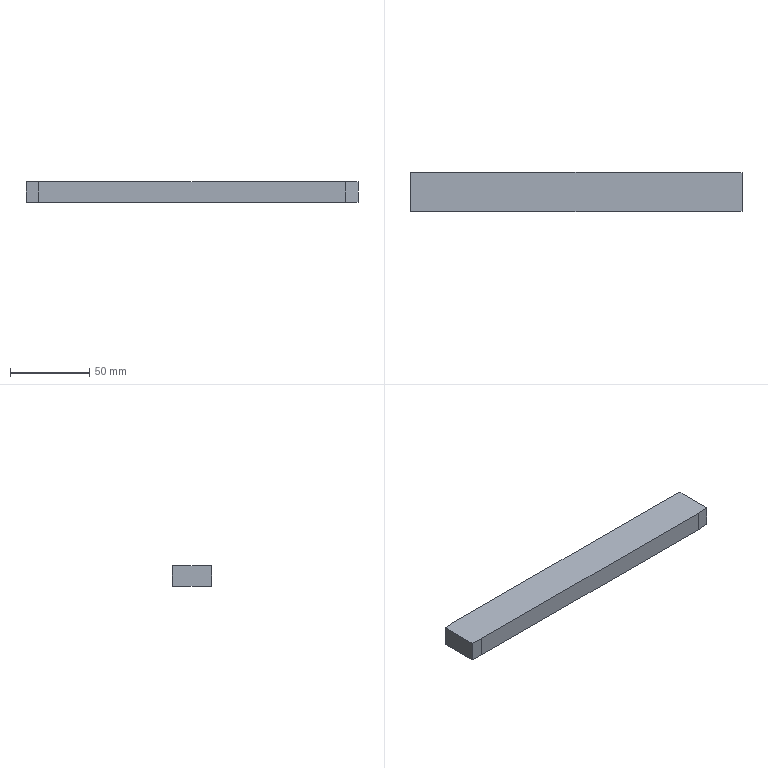Part | SolidWorks | features Cut 1, Extrusion 1 | 1 solid | 10 faces | box 209.55 x 25 x 12.7 mm | volume 66431 mm3 | plane 10
STEP:
#1=CARTESIAN_POINT('',(-104.775,12.,-6.35));
#2=VERTEX_POINT('',#1);
#3=CARTESIAN_POINT('',(-104.775,-12.,-6.35));
#4=VERTEX_POINT('',#3);
#5=CARTESIAN_POINT('',(-104.775,12.5,-6.35));
#6=DIRECTION('',(0.,-1.,0.));
#7=VECTOR('',#6,1000.);
#8=LINE('',#5,#7);
#9=EDGE_CURVE('',#2,#4,#8,.T.);
#10=ORIENTED_EDGE('',*,*,#9,.T.);
#11=CARTESIAN_POINT('',(-104.775,-12.,6.35));
#12=VERTEX_POINT('',#11);
#13=CARTESIAN_POINT('',(-104.775,-12.,-6.35));
#14=DIRECTION('',(0.,0.,1.));
#15=VECTOR('',#14,1000.);
#16=LINE('',#13,#15);
#17=EDGE_CURVE('',#4,#12,#16,.T.);
#18=ORIENTED_EDGE('',*,*,#17,.T.);
#19=CARTESIAN_POINT('',(-104.775,12.,6.35));
#20=VERTEX_POINT('',#19);
#21=CARTESIAN_POINT('',(-104.775,12.5,6.35));
#22=DIRECTION('',(0.,-1.,0.));
#23=VECTOR('',#22,1000.);
#24=LINE('',#21,#23);
#25=EDGE_CURVE('',#20,#12,#24,.T.);
#26=ORIENTED_EDGE('',*,*,#25,.F.);
#27=CARTESIAN_POINT('',(-104.775,12.,-6.35));
#28=DIRECTION('',(0.,0.,1.));
#29=VECTOR('',#28,1000.);
#30=LINE('',#27,#29);
#31=EDGE_CURVE('',#2,#20,#30,.T.);
#32=ORIENTED_EDGE('',*,*,#31,.F.);
#33=EDGE_LOOP('',(#10,#18,#26,#32));
#34=FACE_OUTER_BOUND('',#33,.T.);
#35=CARTESIAN_POINT('',(-104.775,12.5,6.35));
#36=DIRECTION('',(1.,0.,0.));
#37=DIRECTION('',(0.,0.,-1.));
#38=AXIS2_PLACEMENT_3D('',#35,#36,#37);
#39=PLANE('',#38);
#40=ADVANCED_FACE('',(#34),#39,.F.);
#41=CARTESIAN_POINT('',(-96.775,-12.5,6.35));
#42=VERTEX_POINT('',#41);
#43=CARTESIAN_POINT('',(96.775,-12.5,6.35));
#44=VERTEX_POINT('',#43);
#45=CARTESIAN_POINT('',(-104.775,-12.5,6.35));
#46=DIRECTION('',(1.,0.,0.));
#47=VECTOR('',#46,1000.);
#48=LINE('',#45,#47);
#49=EDGE_CURVE('',#42,#44,#48,.T.);
#50=ORIENTED_EDGE('',*,*,#49,.F.);
#51=CARTESIAN_POINT('',(-96.775,-12.5,-6.35));
#52=VERTEX_POINT('',#51);
#53=CARTESIAN_POINT('',(-96.775,-12.5,-6.35));
#54=DIRECTION('',(0.,0.,1.));
#55=VECTOR('',#54,1000.);
#56=LINE('',#53,#55);
#57=EDGE_CURVE('',#52,#42,#56,.T.);
#58=ORIENTED_EDGE('',*,*,#57,.F.);
#59=CARTESIAN_POINT('',(96.775,-12.5,-6.35));
#60=VERTEX_POINT('',#59);
#61=CARTESIAN_POINT('',(-104.775,-12.5,-6.35));
#62=DIRECTION('',(1.,0.,0.));
#63=VECTOR('',#62,1000.);
#64=LINE('',#61,#63);
#65=EDGE_CURVE('',#52,#60,#64,.T.);
#66=ORIENTED_EDGE('',*,*,#65,.T.);
#67=CARTESIAN_POINT('',(96.775,-12.5,-6.35));
#68=DIRECTION('',(0.,0.,1.));
#69=VECTOR('',#68,1000.);
#70=LINE('',#67,#69);
#71=EDGE_CURVE('',#60,#44,#70,.T.);
#72=ORIENTED_EDGE('',*,*,#71,.T.);
#73=EDGE_LOOP('',(#50,#58,#66,#72));
#74=FACE_OUTER_BOUND('',#73,.T.);
#75=CARTESIAN_POINT('',(-104.775,-12.5,6.35));
#76=DIRECTION('',(0.,1.,0.));
#77=DIRECTION('',(-1.,0.,0.));
#78=AXIS2_PLACEMENT_3D('',#75,#76,#77);
#79=PLANE('',#78);
#80=ADVANCED_FACE('',(#74),#79,.F.);
#81=CARTESIAN_POINT('',(104.775,-12.,6.35));
#82=VERTEX_POINT('',#81);
#83=CARTESIAN_POINT('',(104.775,12.,6.35));
#84=VERTEX_POINT('',#83);
#85=CARTESIAN_POINT('',(104.775,12.5,6.35));
#86=DIRECTION('',(0.,1.,0.));
#87=VECTOR('',#86,1000.);
#88=LINE('',#85,#87);
#89=EDGE_CURVE('',#82,#84,#88,.T.);
#90=ORIENTED_EDGE('',*,*,#89,.F.);
#91=CARTESIAN_POINT('',(104.775,-12.,-6.35));
#92=VERTEX_POINT('',#91);
#93=CARTESIAN_POINT('',(104.775,-12.,-6.35));
#94=DIRECTION('',(0.,0.,1.));
#95=VECTOR('',#94,1000.);
#96=LINE('',#93,#95);
#97=EDGE_CURVE('',#92,#82,#96,.T.);
#98=ORIENTED_EDGE('',*,*,#97,.F.);
#99=CARTESIAN_POINT('',(104.775,12.,-6.35));
#100=VERTEX_POINT('',#99);
#101=CARTESIAN_POINT('',(104.775,12.5,-6.35));
#102=DIRECTION('',(0.,1.,0.));
#103=VECTOR('',#102,1000.);
#104=LINE('',#101,#103);
#105=EDGE_CURVE('',#92,#100,#104,.T.);
#106=ORIENTED_EDGE('',*,*,#105,.T.);
#107=CARTESIAN_POINT('',(104.775,12.,-6.35));
#108=DIRECTION('',(0.,0.,1.));
#109=VECTOR('',#108,1000.);
#110=LINE('',#107,#109);
#111=EDGE_CURVE('',#100,#84,#110,.T.);
#112=ORIENTED_EDGE('',*,*,#111,.T.);
#113=EDGE_LOOP('',(#90,#98,#106,#112));
#114=FACE_OUTER_BOUND('',#113,.T.);
#115=CARTESIAN_POINT('',(104.775,12.5,6.35));
#116=DIRECTION('',(-1.,0.,0.));
#117=DIRECTION('',(0.,0.,1.));
#118=AXIS2_PLACEMENT_3D('',#115,#116,#117);
#119=PLANE('',#118);
#120=ADVANCED_FACE('',(#114),#119,.F.);
#121=CARTESIAN_POINT('',(96.775,12.5,6.35));
#122=VERTEX_POINT('',#121);
#123=CARTESIAN_POINT('',(-96.775,12.5,6.35));
#124=VERTEX_POINT('',#123);
#125=CARTESIAN_POINT('',(-104.775,12.5,6.35));
#126=DIRECTION('',(-1.,0.,0.));
#127=VECTOR('',#126,1000.);
#128=LINE('',#125,#127);
#129=EDGE_CURVE('',#122,#124,#128,.T.);
#130=ORIENTED_EDGE('',*,*,#129,.F.);
#131=CARTESIAN_POINT('',(96.775,12.5,-6.35));
#132=VERTEX_POINT('',#131);
#133=CARTESIAN_POINT('',(96.775,12.5,-6.35));
#134=DIRECTION('',(0.,0.,1.));
#135=VECTOR('',#134,1000.);
#136=LINE('',#133,#135);
#137=EDGE_CURVE('',#132,#122,#136,.T.);
#138=ORIENTED_EDGE('',*,*,#137,.F.);
#139=CARTESIAN_POINT('',(-96.775,12.5,-6.35));
#140=VERTEX_POINT('',#139);
#141=CARTESIAN_POINT('',(-104.775,12.5,-6.35));
#142=DIRECTION('',(-1.,0.,0.));
#143=VECTOR('',#142,1000.);
#144=LINE('',#141,#143);
#145=EDGE_CURVE('',#132,#140,#144,.T.);
#146=ORIENTED_EDGE('',*,*,#145,.T.);
#147=CARTESIAN_POINT('',(-96.775,12.5,-6.35));
#148=DIRECTION('',(0.,0.,1.));
#149=VECTOR('',#148,1000.);
#150=LINE('',#147,#149);
#151=EDGE_CURVE('',#140,#124,#150,.T.);
#152=ORIENTED_EDGE('',*,*,#151,.T.);
#153=EDGE_LOOP('',(#130,#138,#146,#152));
#154=FACE_OUTER_BOUND('',#153,.T.);
#155=CARTESIAN_POINT('',(-104.775,12.5,6.35));
#156=DIRECTION('',(0.,-1.,0.));
#157=DIRECTION('',(1.,0.,0.));
#158=AXIS2_PLACEMENT_3D('',#155,#156,#157);
#159=PLANE('',#158);
#160=ADVANCED_FACE('',(#154),#159,.F.);
#161=CARTESIAN_POINT('',(-104.775,-12.,6.35));
#162=DIRECTION('',(-0.9981,0.06238,0.));
#163=VECTOR('',#162,1000.);
#164=LINE('',#161,#163);
#165=EDGE_CURVE('',#42,#12,#164,.T.);
#166=ORIENTED_EDGE('',*,*,#165,.F.);
#167=ORIENTED_EDGE('',*,*,#49,.T.);
#168=CARTESIAN_POINT('',(104.775,-12.,6.35));
#169=DIRECTION('',(-0.9981,-0.06238,0.));
#170=VECTOR('',#169,1000.);
#171=LINE('',#168,#170);
#172=EDGE_CURVE('',#82,#44,#171,.T.);
#173=ORIENTED_EDGE('',*,*,#172,.F.);
#174=ORIENTED_EDGE('',*,*,#89,.T.);
#175=CARTESIAN_POINT('',(104.775,12.,6.35));
#176=DIRECTION('',(0.9981,-0.06238,0.));
#177=VECTOR('',#176,1000.);
#178=LINE('',#175,#177);
#179=EDGE_CURVE('',#122,#84,#178,.T.);
#180=ORIENTED_EDGE('',*,*,#179,.F.);
#181=ORIENTED_EDGE('',*,*,#129,.T.);
#182=CARTESIAN_POINT('',(-104.775,12.,6.35));
#183=DIRECTION('',(0.9981,0.06238,0.));
#184=VECTOR('',#183,1000.);
#185=LINE('',#182,#184);
#186=EDGE_CURVE('',#20,#124,#185,.T.);
#187=ORIENTED_EDGE('',*,*,#186,.F.);
#188=ORIENTED_EDGE('',*,*,#25,.T.);
#189=EDGE_LOOP('',(#166,#167,#173,#174,#180,#181,#187,#188));
#190=FACE_OUTER_BOUND('',#189,.T.);
#191=CARTESIAN_POINT('',(-104.775,-12.5,6.35));
#192=DIRECTION('',(0.,0.,1.));
#193=DIRECTION('',(1.,0.,0.));
#194=AXIS2_PLACEMENT_3D('',#191,#192,#193);
#195=PLANE('',#194);
#196=ADVANCED_FACE('',(#190),#195,.T.);
#197=ORIENTED_EDGE('',*,*,#65,.F.);
#198=CARTESIAN_POINT('',(-104.775,-12.,-6.35));
#199=DIRECTION('',(-0.9981,0.06238,0.));
#200=VECTOR('',#199,1000.);
#201=LINE('',#198,#200);
#202=EDGE_CURVE('',#52,#4,#201,.T.);
#203=ORIENTED_EDGE('',*,*,#202,.T.);
#204=ORIENTED_EDGE('',*,*,#9,.F.);
#205=CARTESIAN_POINT('',(-104.775,12.,-6.35));
#206=DIRECTION('',(0.9981,0.06238,0.));
#207=VECTOR('',#206,1000.);
#208=LINE('',#205,#207);
#209=EDGE_CURVE('',#2,#140,#208,.T.);
#210=ORIENTED_EDGE('',*,*,#209,.T.);
#211=ORIENTED_EDGE('',*,*,#145,.F.);
#212=CARTESIAN_POINT('',(104.775,12.,-6.35));
#213=DIRECTION('',(0.9981,-0.06238,0.));
#214=VECTOR('',#213,1000.);
#215=LINE('',#212,#214);
#216=EDGE_CURVE('',#132,#100,#215,.T.);
#217=ORIENTED_EDGE('',*,*,#216,.T.);
#218=ORIENTED_EDGE('',*,*,#105,.F.);
#219=CARTESIAN_POINT('',(104.775,-12.,-6.35));
#220=DIRECTION('',(-0.9981,-0.06238,0.));
#221=VECTOR('',#220,1000.);
#222=LINE('',#219,#221);
#223=EDGE_CURVE('',#92,#60,#222,.T.);
#224=ORIENTED_EDGE('',*,*,#223,.T.);
#225=EDGE_LOOP('',(#197,#203,#204,#210,#211,#217,#218,#224));
#226=FACE_OUTER_BOUND('',#225,.T.);
#227=CARTESIAN_POINT('',(-104.775,-12.5,-6.35));
#228=DIRECTION('',(0.,0.,1.));
#229=DIRECTION('',(1.,0.,0.));
#230=AXIS2_PLACEMENT_3D('',#227,#228,#229);
#231=PLANE('',#230);
#232=ADVANCED_FACE('',(#226),#231,.F.);
#233=ORIENTED_EDGE('',*,*,#186,.T.);
#234=ORIENTED_EDGE('',*,*,#151,.F.);
#235=ORIENTED_EDGE('',*,*,#209,.F.);
#236=ORIENTED_EDGE('',*,*,#31,.T.);
#237=EDGE_LOOP('',(#233,#234,#235,#236));
#238=FACE_OUTER_BOUND('',#237,.T.);
#239=CARTESIAN_POINT('',(-104.775,12.,-6.35));
#240=DIRECTION('',(0.06238,-0.9981,0.));
#241=DIRECTION('',(0.9981,0.06238,0.));
#242=AXIS2_PLACEMENT_3D('',#239,#240,#241);
#243=PLANE('',#242);
#244=ADVANCED_FACE('',(#238),#243,.F.);
#245=ORIENTED_EDGE('',*,*,#179,.T.);
#246=ORIENTED_EDGE('',*,*,#111,.F.);
#247=ORIENTED_EDGE('',*,*,#216,.F.);
#248=ORIENTED_EDGE('',*,*,#137,.T.);
#249=EDGE_LOOP('',(#245,#246,#247,#248));
#250=FACE_OUTER_BOUND('',#249,.T.);
#251=CARTESIAN_POINT('',(104.775,12.,-6.35));
#252=DIRECTION('',(-0.06238,-0.9981,0.));
#253=DIRECTION('',(0.9981,-0.06238,0.));
#254=AXIS2_PLACEMENT_3D('',#251,#252,#253);
#255=PLANE('',#254);
#256=ADVANCED_FACE('',(#250),#255,.F.);
#257=ORIENTED_EDGE('',*,*,#172,.T.);
#258=ORIENTED_EDGE('',*,*,#71,.F.);
#259=ORIENTED_EDGE('',*,*,#223,.F.);
#260=ORIENTED_EDGE('',*,*,#97,.T.);
#261=EDGE_LOOP('',(#257,#258,#259,#260));
#262=FACE_OUTER_BOUND('',#261,.T.);
#263=CARTESIAN_POINT('',(104.775,-12.,-6.35));
#264=DIRECTION('',(-0.06238,0.9981,0.));
#265=DIRECTION('',(-0.9981,-0.06238,0.));
#266=AXIS2_PLACEMENT_3D('',#263,#264,#265);
#267=PLANE('',#266);
#268=ADVANCED_FACE('',(#262),#267,.F.);
#269=ORIENTED_EDGE('',*,*,#165,.T.);
#270=ORIENTED_EDGE('',*,*,#17,.F.);
#271=ORIENTED_EDGE('',*,*,#202,.F.);
#272=ORIENTED_EDGE('',*,*,#57,.T.);
#273=EDGE_LOOP('',(#269,#270,#271,#272));
#274=FACE_OUTER_BOUND('',#273,.T.);
#275=CARTESIAN_POINT('',(-104.775,-12.,-6.35));
#276=DIRECTION('',(0.06238,0.9981,0.));
#277=DIRECTION('',(-0.9981,0.06238,0.));
#278=AXIS2_PLACEMENT_3D('',#275,#276,#277);
#279=PLANE('',#278);
#280=ADVANCED_FACE('',(#274),#279,.F.);
#281=CLOSED_SHELL('',(#40,#80,#120,#160,#196,#232,#244,#256,#268,#280));
#282=MANIFOLD_SOLID_BREP('',#281);
#283=CARTESIAN_POINT('',(0.,0.,0.));
#284=DIRECTION('',(0.,0.,1.));
#285=DIRECTION('',(1.,0.,0.));
#286=AXIS2_PLACEMENT_3D('',#283,#284,#285);
#287=(LENGTH_UNIT()NAMED_UNIT(*)SI_UNIT(.MILLI.,.METRE.));
#288=UNCERTAINTY_MEASURE_WITH_UNIT(LENGTH_MEASURE(0.00001),#287,'','');
#289=(NAMED_UNIT(*)PLANE_ANGLE_UNIT()SI_UNIT($,.RADIAN.));
#290=(NAMED_UNIT(*)SI_UNIT($,.STERADIAN.)SOLID_ANGLE_UNIT());
#291=(GEOMETRIC_REPRESENTATION_CONTEXT(3)GLOBAL_UNCERTAINTY_ASSIGNED_CONTEXT((#288))GLOBAL_UNIT_ASSIGNED_CONTEXT((#287,#289,#290))REPRESENTATION_CONTEXT('',''));
#292=ADVANCED_BREP_SHAPE_REPRESENTATION('',(#282,#286),#291);